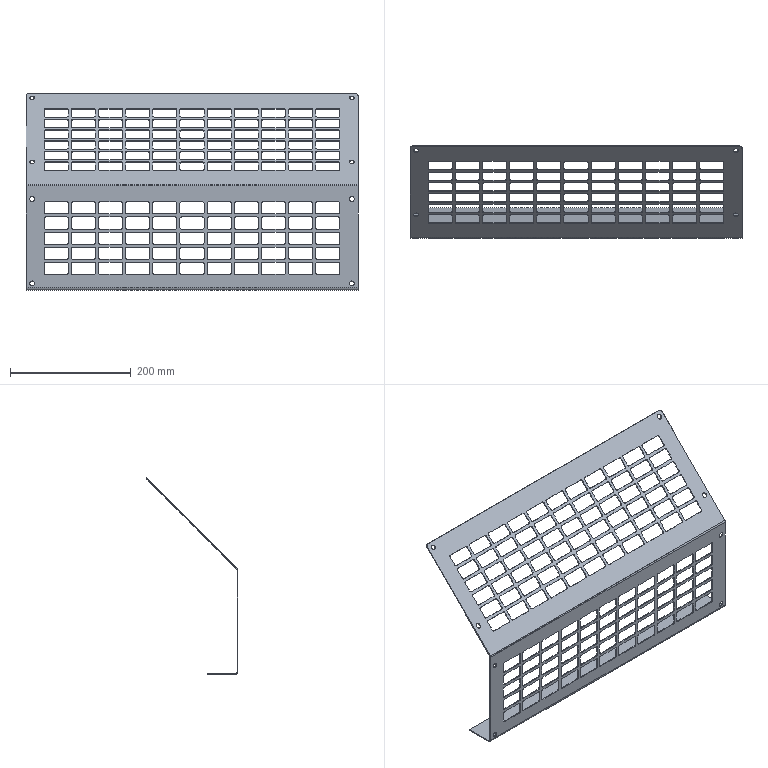Part | STEP file | SYL_0392D6J1SYL0380DJ100-149154 | 1 solid | 1008 faces | box 550 x 152.382 x 325.821 mm | volume 213564 mm3 | cylinder 506 | plane 502 | commonest cylinder face diameters 5 x484 8 x16 10 x3 7 x2 4 x1